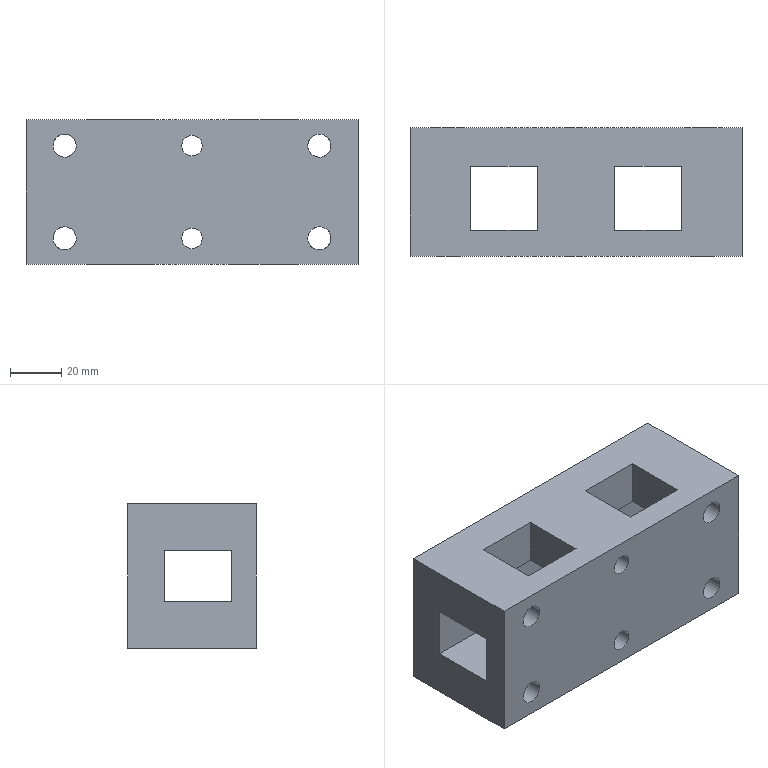Part | STEP file | 车灯-后视镜_id42_x_t | 1 solid | 40 faces | box 129 x 50 x 56 mm | volume 226318 mm3 | plane 30 | cylinder 10 | commonest cylinder face diameters 9 x4 14 x4 8 x2
STEP:
#1=CARTESIAN_POINT('',(65.5,310.,-247.5));
#2=VERTEX_POINT('',#1);
#3=CARTESIAN_POINT('',(65.5,310.,-229.5));
#4=VERTEX_POINT('',#3);
#5=CARTESIAN_POINT('',(65.5,310.,-335.5));
#6=DIRECTION('',(0.,0.,1.));
#7=VECTOR('',#6,1.);
#8=LINE('',#5,#7);
#9=EDGE_CURVE('',#2,#4,#8,.T.);
#10=ORIENTED_EDGE('',*,*,#9,.F.);
#11=CARTESIAN_POINT('',(65.5,285.,-247.5));
#12=VERTEX_POINT('',#11);
#13=CARTESIAN_POINT('',(65.5,292.5,-247.5));
#14=DIRECTION('',(0.,-1.,0.));
#15=VECTOR('',#14,1.);
#16=LINE('',#13,#15);
#17=EDGE_CURVE('',#2,#12,#16,.T.);
#18=ORIENTED_EDGE('',*,*,#17,.T.);
#19=CARTESIAN_POINT('',(65.5,285.,-229.5));
#20=VERTEX_POINT('',#19);
#21=CARTESIAN_POINT('',(65.5,285.,-335.5));
#22=DIRECTION('',(0.,0.,1.));
#23=VECTOR('',#22,1.);
#24=LINE('',#21,#23);
#25=EDGE_CURVE('',#12,#20,#24,.T.);
#26=ORIENTED_EDGE('',*,*,#25,.T.);
#27=CARTESIAN_POINT('',(65.5,292.5,-229.5));
#28=DIRECTION('',(0.,1.,0.));
#29=VECTOR('',#28,1.);
#30=LINE('',#27,#29);
#31=EDGE_CURVE('',#20,#4,#30,.T.);
#32=ORIENTED_EDGE('',*,*,#31,.T.);
#33=EDGE_LOOP('',(#10,#18,#26,#32));
#34=FACE_OUTER_BOUND('',#33,.T.);
#35=CARTESIAN_POINT('',(65.5,292.5,-335.5));
#36=DIRECTION('',(1.,0.,0.));
#37=DIRECTION('',(0.,0.,-1.));
#38=AXIS2_PLACEMENT_3D('',#35,#36,#37);
#39=PLANE('',#38);
#40=ADVANCED_FACE('',(#34),#39,.F.);
#41=ORIENTED_EDGE('',*,*,#25,.F.);
#42=CARTESIAN_POINT('',(39.5,285.,-247.5));
#43=VERTEX_POINT('',#42);
#44=CARTESIAN_POINT('',(52.5,285.,-247.5));
#45=DIRECTION('',(-1.,0.,0.));
#46=VECTOR('',#45,1.);
#47=LINE('',#44,#46);
#48=EDGE_CURVE('',#12,#43,#47,.T.);
#49=ORIENTED_EDGE('',*,*,#48,.T.);
#50=CARTESIAN_POINT('',(39.5,285.,-229.5));
#51=VERTEX_POINT('',#50);
#52=CARTESIAN_POINT('',(39.5,285.,-335.5));
#53=DIRECTION('',(0.,0.,1.));
#54=VECTOR('',#53,1.);
#55=LINE('',#52,#54);
#56=EDGE_CURVE('',#43,#51,#55,.T.);
#57=ORIENTED_EDGE('',*,*,#56,.T.);
#58=CARTESIAN_POINT('',(52.5,285.,-229.5));
#59=DIRECTION('',(1.,0.,0.));
#60=VECTOR('',#59,1.);
#61=LINE('',#58,#60);
#62=EDGE_CURVE('',#51,#20,#61,.T.);
#63=ORIENTED_EDGE('',*,*,#62,.T.);
#64=EDGE_LOOP('',(#41,#49,#57,#63));
#65=FACE_OUTER_BOUND('',#64,.T.);
#66=CARTESIAN_POINT('',(52.5,285.,-335.5));
#67=DIRECTION('',(0.,-1.,0.));
#68=DIRECTION('',(0.,0.,1.));
#69=AXIS2_PLACEMENT_3D('',#66,#67,#68);
#70=PLANE('',#69);
#71=ADVANCED_FACE('',(#65),#70,.F.);
#72=ORIENTED_EDGE('',*,*,#56,.F.);
#73=CARTESIAN_POINT('',(39.5,310.,-247.5));
#74=VERTEX_POINT('',#73);
#75=CARTESIAN_POINT('',(39.5,292.5,-247.5));
#76=DIRECTION('',(0.,1.,0.));
#77=VECTOR('',#76,1.);
#78=LINE('',#75,#77);
#79=EDGE_CURVE('',#43,#74,#78,.T.);
#80=ORIENTED_EDGE('',*,*,#79,.T.);
#81=CARTESIAN_POINT('',(39.5,310.,-229.5));
#82=VERTEX_POINT('',#81);
#83=CARTESIAN_POINT('',(39.5,310.,-335.5));
#84=DIRECTION('',(0.,0.,1.));
#85=VECTOR('',#84,1.);
#86=LINE('',#83,#85);
#87=EDGE_CURVE('',#74,#82,#86,.T.);
#88=ORIENTED_EDGE('',*,*,#87,.T.);
#89=CARTESIAN_POINT('',(39.5,292.5,-229.5));
#90=DIRECTION('',(0.,-1.,0.));
#91=VECTOR('',#90,1.);
#92=LINE('',#89,#91);
#93=EDGE_CURVE('',#82,#51,#92,.T.);
#94=ORIENTED_EDGE('',*,*,#93,.T.);
#95=EDGE_LOOP('',(#72,#80,#88,#94));
#96=FACE_OUTER_BOUND('',#95,.T.);
#97=CARTESIAN_POINT('',(39.5,292.5,-335.5));
#98=DIRECTION('',(-1.,0.,0.));
#99=DIRECTION('',(0.,0.,1.));
#100=AXIS2_PLACEMENT_3D('',#97,#98,#99);
#101=PLANE('',#100);
#102=ADVANCED_FACE('',(#96),#101,.F.);
#103=ORIENTED_EDGE('',*,*,#87,.F.);
#104=CARTESIAN_POINT('',(52.5,310.,-247.5));
#105=DIRECTION('',(1.,0.,0.));
#106=VECTOR('',#105,1.);
#107=LINE('',#104,#106);
#108=EDGE_CURVE('',#74,#2,#107,.T.);
#109=ORIENTED_EDGE('',*,*,#108,.T.);
#110=ORIENTED_EDGE('',*,*,#9,.T.);
#111=CARTESIAN_POINT('',(52.5,310.,-229.5));
#112=DIRECTION('',(-1.,0.,0.));
#113=VECTOR('',#112,1.);
#114=LINE('',#111,#113);
#115=EDGE_CURVE('',#4,#82,#114,.T.);
#116=ORIENTED_EDGE('',*,*,#115,.T.);
#117=EDGE_LOOP('',(#103,#109,#110,#116));
#118=FACE_OUTER_BOUND('',#117,.T.);
#119=CARTESIAN_POINT('',(52.5,310.,-335.5));
#120=DIRECTION('',(0.,1.,0.));
#121=DIRECTION('',(0.,0.,-1.));
#122=AXIS2_PLACEMENT_3D('',#119,#120,#121);
#123=PLANE('',#122);
#124=ADVANCED_FACE('',(#118),#123,.F.);
#125=CARTESIAN_POINT('',(121.5,310.,-247.5));
#126=VERTEX_POINT('',#125);
#127=CARTESIAN_POINT('',(121.5,310.,-229.5));
#128=VERTEX_POINT('',#127);
#129=CARTESIAN_POINT('',(121.5,310.,-335.5));
#130=DIRECTION('',(0.,0.,1.));
#131=VECTOR('',#130,1.);
#132=LINE('',#129,#131);
#133=EDGE_CURVE('',#126,#128,#132,.T.);
#134=ORIENTED_EDGE('',*,*,#133,.F.);
#135=CARTESIAN_POINT('',(121.5,285.,-247.5));
#136=VERTEX_POINT('',#135);
#137=CARTESIAN_POINT('',(121.5,292.5,-247.5));
#138=DIRECTION('',(0.,-1.,0.));
#139=VECTOR('',#138,1.);
#140=LINE('',#137,#139);
#141=EDGE_CURVE('',#126,#136,#140,.T.);
#142=ORIENTED_EDGE('',*,*,#141,.T.);
#143=CARTESIAN_POINT('',(121.5,285.,-229.5));
#144=VERTEX_POINT('',#143);
#145=CARTESIAN_POINT('',(121.5,285.,-335.5));
#146=DIRECTION('',(0.,0.,1.));
#147=VECTOR('',#146,1.);
#148=LINE('',#145,#147);
#149=EDGE_CURVE('',#136,#144,#148,.T.);
#150=ORIENTED_EDGE('',*,*,#149,.T.);
#151=CARTESIAN_POINT('',(121.5,292.5,-229.5));
#152=DIRECTION('',(0.,1.,0.));
#153=VECTOR('',#152,1.);
#154=LINE('',#151,#153);
#155=EDGE_CURVE('',#144,#128,#154,.T.);
#156=ORIENTED_EDGE('',*,*,#155,.T.);
#157=EDGE_LOOP('',(#134,#142,#150,#156));
#158=FACE_OUTER_BOUND('',#157,.T.);
#159=CARTESIAN_POINT('',(121.5,292.5,-335.5));
#160=DIRECTION('',(1.,0.,0.));
#161=DIRECTION('',(0.,0.,-1.));
#162=AXIS2_PLACEMENT_3D('',#159,#160,#161);
#163=PLANE('',#162);
#164=ADVANCED_FACE('',(#158),#163,.F.);
#165=ORIENTED_EDGE('',*,*,#149,.F.);
#166=CARTESIAN_POINT('',(95.5,285.,-247.5));
#167=VERTEX_POINT('',#166);
#168=CARTESIAN_POINT('',(108.5,285.,-247.5));
#169=DIRECTION('',(-1.,0.,0.));
#170=VECTOR('',#169,1.);
#171=LINE('',#168,#170);
#172=EDGE_CURVE('',#136,#167,#171,.T.);
#173=ORIENTED_EDGE('',*,*,#172,.T.);
#174=CARTESIAN_POINT('',(95.5,285.,-229.5));
#175=VERTEX_POINT('',#174);
#176=CARTESIAN_POINT('',(95.5,285.,-335.5));
#177=DIRECTION('',(0.,0.,1.));
#178=VECTOR('',#177,1.);
#179=LINE('',#176,#178);
#180=EDGE_CURVE('',#167,#175,#179,.T.);
#181=ORIENTED_EDGE('',*,*,#180,.T.);
#182=CARTESIAN_POINT('',(108.5,285.,-229.5));
#183=DIRECTION('',(1.,0.,0.));
#184=VECTOR('',#183,1.);
#185=LINE('',#182,#184);
#186=EDGE_CURVE('',#175,#144,#185,.T.);
#187=ORIENTED_EDGE('',*,*,#186,.T.);
#188=EDGE_LOOP('',(#165,#173,#181,#187));
#189=FACE_OUTER_BOUND('',#188,.T.);
#190=CARTESIAN_POINT('',(108.5,285.,-335.5));
#191=DIRECTION('',(0.,-1.,0.));
#192=DIRECTION('',(0.,0.,1.));
#193=AXIS2_PLACEMENT_3D('',#190,#191,#192);
#194=PLANE('',#193);
#195=ADVANCED_FACE('',(#189),#194,.F.);
#196=ORIENTED_EDGE('',*,*,#180,.F.);
#197=CARTESIAN_POINT('',(95.5,310.,-247.5));
#198=VERTEX_POINT('',#197);
#199=CARTESIAN_POINT('',(95.5,292.5,-247.5));
#200=DIRECTION('',(0.,1.,0.));
#201=VECTOR('',#200,1.);
#202=LINE('',#199,#201);
#203=EDGE_CURVE('',#167,#198,#202,.T.);
#204=ORIENTED_EDGE('',*,*,#203,.T.);
#205=CARTESIAN_POINT('',(95.5,310.,-229.5));
#206=VERTEX_POINT('',#205);
#207=CARTESIAN_POINT('',(95.5,310.,-335.5));
#208=DIRECTION('',(0.,0.,1.));
#209=VECTOR('',#208,1.);
#210=LINE('',#207,#209);
#211=EDGE_CURVE('',#198,#206,#210,.T.);
#212=ORIENTED_EDGE('',*,*,#211,.T.);
#213=CARTESIAN_POINT('',(95.5,300.,-229.5));
#214=DIRECTION('',(0.,1.,0.));
#215=VECTOR('',#214,1.);
#216=LINE('',#213,#215);
#217=EDGE_CURVE('',#175,#206,#216,.T.);
#218=ORIENTED_EDGE('',*,*,#217,.F.);
#219=EDGE_LOOP('',(#196,#204,#212,#218));
#220=FACE_OUTER_BOUND('',#219,.T.);
#221=CARTESIAN_POINT('',(95.5,292.5,-335.5));
#222=DIRECTION('',(-1.,0.,0.));
#223=DIRECTION('',(0.,0.,1.));
#224=AXIS2_PLACEMENT_3D('',#221,#222,#223);
#225=PLANE('',#224);
#226=ADVANCED_FACE('',(#220),#225,.F.);
#227=ORIENTED_EDGE('',*,*,#211,.F.);
#228=CARTESIAN_POINT('',(108.5,310.,-247.5));
#229=DIRECTION('',(1.,0.,0.));
#230=VECTOR('',#229,1.);
#231=LINE('',#228,#230);
#232=EDGE_CURVE('',#198,#126,#231,.T.);
#233=ORIENTED_EDGE('',*,*,#232,.T.);
#234=ORIENTED_EDGE('',*,*,#133,.T.);
#235=CARTESIAN_POINT('',(108.5,310.,-229.5));
#236=DIRECTION('',(-1.,0.,0.));
#237=VECTOR('',#236,1.);
#238=LINE('',#235,#237);
#239=EDGE_CURVE('',#128,#206,#238,.T.);
#240=ORIENTED_EDGE('',*,*,#239,.T.);
#241=EDGE_LOOP('',(#227,#233,#234,#240));
#242=FACE_OUTER_BOUND('',#241,.T.);
#243=CARTESIAN_POINT('',(108.5,310.,-335.5));
#244=DIRECTION('',(0.,1.,0.));
#245=DIRECTION('',(0.,0.,-1.));
#246=AXIS2_PLACEMENT_3D('',#243,#244,#245);
#247=PLANE('',#246);
#248=ADVANCED_FACE('',(#242),#247,.F.);
#249=ORIENTED_EDGE('',*,*,#155,.F.);
#250=ORIENTED_EDGE('',*,*,#186,.F.);
#251=ORIENTED_EDGE('',*,*,#217,.T.);
#252=ORIENTED_EDGE('',*,*,#239,.F.);
#253=EDGE_LOOP('',(#249,#250,#251,#252));
#254=FACE_BOUND('',#253,.T.);
#255=ORIENTED_EDGE('',*,*,#31,.F.);
#256=ORIENTED_EDGE('',*,*,#62,.F.);
#257=ORIENTED_EDGE('',*,*,#93,.F.);
#258=ORIENTED_EDGE('',*,*,#115,.F.);
#259=EDGE_LOOP('',(#255,#256,#257,#258));
#260=FACE_BOUND('',#259,.T.);
#261=CARTESIAN_POINT('',(16.,325.,-229.5));
#262=VERTEX_POINT('',#261);
#263=CARTESIAN_POINT('',(145.,325.,-229.5));
#264=VERTEX_POINT('',#263);
#265=CARTESIAN_POINT('',(80.5,325.,-229.5));
#266=DIRECTION('',(1.,0.,0.));
#267=VECTOR('',#266,1.);
#268=LINE('',#265,#267);
#269=EDGE_CURVE('',#262,#264,#268,.T.);
#270=ORIENTED_EDGE('',*,*,#269,.F.);
#271=CARTESIAN_POINT('',(16.,275.,-229.5));
#272=VERTEX_POINT('',#271);
#273=CARTESIAN_POINT('',(16.,300.,-229.5));
#274=DIRECTION('',(0.,1.,0.));
#275=VECTOR('',#274,1.);
#276=LINE('',#273,#275);
#277=EDGE_CURVE('',#272,#262,#276,.T.);
#278=ORIENTED_EDGE('',*,*,#277,.F.);
#279=CARTESIAN_POINT('',(145.,275.,-229.5));
#280=VERTEX_POINT('',#279);
#281=CARTESIAN_POINT('',(80.5,275.,-229.5));
#282=DIRECTION('',(-1.,0.,0.));
#283=VECTOR('',#282,1.);
#284=LINE('',#281,#283);
#285=EDGE_CURVE('',#280,#272,#284,.T.);
#286=ORIENTED_EDGE('',*,*,#285,.F.);
#287=CARTESIAN_POINT('',(145.,300.,-229.5));
#288=DIRECTION('',(0.,-1.,0.));
#289=VECTOR('',#288,1.);
#290=LINE('',#287,#289);
#291=EDGE_CURVE('',#264,#280,#290,.T.);
#292=ORIENTED_EDGE('',*,*,#291,.F.);
#293=EDGE_LOOP('',(#270,#278,#286,#292));
#294=FACE_BOUND('',#293,.T.);
#295=CARTESIAN_POINT('',(80.5,300.,-229.5));
#296=DIRECTION('',(0.,0.,1.));
#297=DIRECTION('',(-1.,0.,0.));
#298=AXIS2_PLACEMENT_3D('',#295,#296,#297);
#299=PLANE('',#298);
#300=ADVANCED_FACE('',(#254,#260,#294),#299,.T.);
#301=CARTESIAN_POINT('',(123.,325.,-239.5));
#302=VERTEX_POINT('',#301);
#303=CARTESIAN_POINT('',(130.,325.,-239.5));
#304=DIRECTION('',(0.,-1.,0.));
#305=DIRECTION('',(-1.,0.,0.));
#306=AXIS2_PLACEMENT_3D('',#303,#304,#305);
#307=CIRCLE('',#306,7.);
#308=EDGE_CURVE('',#302,#302,#307,.T.);
#309=ORIENTED_EDGE('',*,*,#308,.T.);
#310=EDGE_LOOP('',(#309));
#311=FACE_BOUND('',#310,.T.);
#312=CARTESIAN_POINT('',(123.,325.,-275.5));
#313=VERTEX_POINT('',#312);
#314=CARTESIAN_POINT('',(130.,325.,-275.5));
#315=DIRECTION('',(0.,-1.,0.));
#316=DIRECTION('',(-1.,0.,0.));
#317=AXIS2_PLACEMENT_3D('',#314,#315,#316);
#318=CIRCLE('',#317,7.);
#319=EDGE_CURVE('',#313,#313,#318,.T.);
#320=ORIENTED_EDGE('',*,*,#319,.T.);
#321=EDGE_LOOP('',(#320));
#322=FACE_BOUND('',#321,.T.);
#323=CARTESIAN_POINT('',(24.,325.,-275.5));
#324=VERTEX_POINT('',#323);
#325=CARTESIAN_POINT('',(31.,325.,-275.5));
#326=DIRECTION('',(0.,-1.,0.));
#327=DIRECTION('',(-1.,0.,0.));
#328=AXIS2_PLACEMENT_3D('',#325,#326,#327);
#329=CIRCLE('',#328,7.);
#330=EDGE_CURVE('',#324,#324,#329,.T.);
#331=ORIENTED_EDGE('',*,*,#330,.T.);
#332=EDGE_LOOP('',(#331));
#333=FACE_BOUND('',#332,.T.);
#334=CARTESIAN_POINT('',(24.,325.,-239.5));
#335=VERTEX_POINT('',#334);
#336=CARTESIAN_POINT('',(31.,325.,-239.5));
#337=DIRECTION('',(0.,-1.,0.));
#338=DIRECTION('',(-1.,0.,0.));
#339=AXIS2_PLACEMENT_3D('',#336,#337,#338);
#340=CIRCLE('',#339,7.);
#341=EDGE_CURVE('',#335,#335,#340,.T.);
#342=ORIENTED_EDGE('',*,*,#341,.T.);
#343=EDGE_LOOP('',(#342));
#344=FACE_BOUND('',#343,.T.);
#345=CARTESIAN_POINT('',(80.5,325.,-271.5));
#346=VERTEX_POINT('',#345);
#347=CARTESIAN_POINT('',(80.5,325.,-275.5));
#348=DIRECTION('',(0.,-1.,0.));
#349=DIRECTION('',(0.,0.,1.));
#350=AXIS2_PLACEMENT_3D('',#347,#348,#349);
#351=CIRCLE('',#350,4.);
#352=EDGE_CURVE('',#346,#346,#351,.T.);
#353=ORIENTED_EDGE('',*,*,#352,.T.);
#354=EDGE_LOOP('',(#353));
#355=FACE_BOUND('',#354,.T.);
#356=CARTESIAN_POINT('',(80.5,325.,-235.5));
#357=VERTEX_POINT('',#356);
#358=CARTESIAN_POINT('',(80.5,325.,-239.5));
#359=DIRECTION('',(0.,-1.,0.));
#360=DIRECTION('',(0.,0.,1.));
#361=AXIS2_PLACEMENT_3D('',#358,#359,#360);
#362=CIRCLE('',#361,4.);
#363=EDGE_CURVE('',#357,#357,#362,.T.);
#364=ORIENTED_EDGE('',*,*,#363,.T.);
#365=EDGE_LOOP('',(#364));
#366=FACE_BOUND('',#365,.T.);
#367=CARTESIAN_POINT('',(16.,325.,-285.5));
#368=VERTEX_POINT('',#367);
#369=CARTESIAN_POINT('',(16.,325.,-285.5));
#370=DIRECTION('',(0.,0.,1.));
#371=VECTOR('',#370,1.);
#372=LINE('',#369,#371);
#373=EDGE_CURVE('',#368,#262,#372,.T.);
#374=ORIENTED_EDGE('',*,*,#373,.T.);
#375=ORIENTED_EDGE('',*,*,#269,.T.);
#376=CARTESIAN_POINT('',(145.,325.,-285.5));
#377=VERTEX_POINT('',#376);
#378=CARTESIAN_POINT('',(145.,325.,-285.5));
#379=DIRECTION('',(0.,0.,1.));
#380=VECTOR('',#379,1.);
#381=LINE('',#378,#380);
#382=EDGE_CURVE('',#377,#264,#381,.T.);
#383=ORIENTED_EDGE('',*,*,#382,.F.);
#384=CARTESIAN_POINT('',(80.5,325.,-285.5));
#385=DIRECTION('',(-1.,0.,0.));
#386=VECTOR('',#385,1.);
#387=LINE('',#384,#386);
#388=EDGE_CURVE('',#377,#368,#387,.T.);
#389=ORIENTED_EDGE('',*,*,#388,.T.);
#390=EDGE_LOOP('',(#374,#375,#383,#389));
#391=FACE_BOUND('',#390,.T.);
#392=CARTESIAN_POINT('',(80.5,325.,-285.5));
#393=DIRECTION('',(0.,1.,0.));
#394=DIRECTION('',(0.,0.,-1.));
#395=AXIS2_PLACEMENT_3D('',#392,#393,#394);
#396=PLANE('',#395);
#397=ADVANCED_FACE('',(#311,#322,#333,#344,#355,#366,#391),#396,.T.);
#398=CARTESIAN_POINT('',(145.,310.5,-247.5));
#399=VERTEX_POINT('',#398);
#400=CARTESIAN_POINT('',(145.,284.5,-247.5));
#401=VERTEX_POINT('',#400);
#402=CARTESIAN_POINT('',(145.,295.,-247.5));
#403=DIRECTION('',(0.,-1.,0.));
#404=VECTOR('',#403,1.);
#405=LINE('',#402,#404);
#406=EDGE_CURVE('',#399,#401,#405,.T.);
#407=ORIENTED_EDGE('',*,*,#406,.F.);
#408=CARTESIAN_POINT('',(145.,310.5,-267.5));
#409=VERTEX_POINT('',#408);
#410=CARTESIAN_POINT('',(145.,310.5,-268.));
#411=DIRECTION('',(0.,0.,1.));
#412=VECTOR('',#411,1.);
#413=LINE('',#410,#412);
#414=EDGE_CURVE('',#409,#399,#413,.T.);
#415=ORIENTED_EDGE('',*,*,#414,.F.);
#416=CARTESIAN_POINT('',(145.,284.5,-267.5));
#417=VERTEX_POINT('',#416);
#418=CARTESIAN_POINT('',(145.,295.,-267.5));
#419=DIRECTION('',(0.,1.,0.));
#420=VECTOR('',#419,1.);
#421=LINE('',#418,#420);
#422=EDGE_CURVE('',#417,#409,#421,.T.);
#423=ORIENTED_EDGE('',*,*,#422,.F.);
#424=CARTESIAN_POINT('',(145.,284.5,-268.));
#425=DIRECTION('',(0.,0.,1.));
#426=VECTOR('',#425,1.);
#427=LINE('',#424,#426);
#428=EDGE_CURVE('',#417,#401,#427,.T.);
#429=ORIENTED_EDGE('',*,*,#428,.T.);
#430=EDGE_LOOP('',(#407,#415,#423,#429));
#431=FACE_BOUND('',#430,.T.);
#432=ORIENTED_EDGE('',*,*,#382,.T.);
#433=ORIENTED_EDGE('',*,*,#291,.T.);
#434=CARTESIAN_POINT('',(145.,275.,-285.5));
#435=VERTEX_POINT('',#434);
#436=CARTESIAN_POINT('',(145.,275.,-285.5));
#437=DIRECTION('',(0.,0.,1.));
#438=VECTOR('',#437,1.);
#439=LINE('',#436,#438);
#440=EDGE_CURVE('',#435,#280,#439,.T.);
#441=ORIENTED_EDGE('',*,*,#440,.F.);
#442=CARTESIAN_POINT('',(145.,300.,-285.5));
#443=DIRECTION('',(0.,1.,0.));
#444=VECTOR('',#443,1.);
#445=LINE('',#442,#444);
#446=EDGE_CURVE('',#435,#377,#445,.T.);
#447=ORIENTED_EDGE('',*,*,#446,.T.);
#448=EDGE_LOOP('',(#432,#433,#441,#447));
#449=FACE_BOUND('',#448,.T.);
#450=CARTESIAN_POINT('',(145.,300.,-285.5));
#451=DIRECTION('',(1.,0.,0.));
#452=DIRECTION('',(0.,0.,1.));
#453=AXIS2_PLACEMENT_3D('',#450,#451,#452);
#454=PLANE('',#453);
#455=ADVANCED_FACE('',(#431,#449),#454,.T.);
#456=CARTESIAN_POINT('',(125.5,275.,-239.5));
#457=VERTEX_POINT('',#456);
#458=CARTESIAN_POINT('',(130.,275.,-239.5));
#459=DIRECTION('',(0.,1.,0.));
#460=DIRECTION('',(-1.,0.,0.));
#461=AXIS2_PLACEMENT_3D('',#458,#459,#460);
#462=CIRCLE('',#461,4.5);
#463=EDGE_CURVE('',#457,#457,#462,.T.);
#464=ORIENTED_EDGE('',*,*,#463,.T.);
#465=EDGE_LOOP('',(#464));
#466=FACE_BOUND('',#465,.T.);
#467=CARTESIAN_POINT('',(125.5,275.,-275.5));
#468=VERTEX_POINT('',#467);
#469=CARTESIAN_POINT('',(130.,275.,-275.5));
#470=DIRECTION('',(0.,1.,0.));
#471=DIRECTION('',(-1.,0.,0.));
#472=AXIS2_PLACEMENT_3D('',#469,#470,#471);
#473=CIRCLE('',#472,4.5);
#474=EDGE_CURVE('',#468,#468,#473,.T.);
#475=ORIENTED_EDGE('',*,*,#474,.T.);
#476=EDGE_LOOP('',(#475));
#477=FACE_BOUND('',#476,.T.);
#478=CARTESIAN_POINT('',(26.5,275.,-275.5));
#479=VERTEX_POINT('',#478);
#480=CARTESIAN_POINT('',(31.,275.,-275.5));
#481=DIRECTION('',(0.,1.,0.));
#482=DIRECTION('',(-1.,0.,0.));
#483=AXIS2_PLACEMENT_3D('',#480,#481,#482);
#484=CIRCLE('',#483,4.5);
#485=EDGE_CURVE('',#479,#479,#484,.T.);
#486=ORIENTED_EDGE('',*,*,#485,.T.);
#487=EDGE_LOOP('',(#486));
#488=FACE_BOUND('',#487,.T.);
#489=CARTESIAN_POINT('',(26.5,275.,-239.5));
#490=VERTEX_POINT('',#489);
#491=CARTESIAN_POINT('',(31.,275.,-239.5));
#492=DIRECTION('',(0.,1.,0.));
#493=DIRECTION('',(-1.,0.,0.));
#494=AXIS2_PLACEMENT_3D('',#491,#492,#493);
#495=CIRCLE('',#494,4.5);
#496=EDGE_CURVE('',#490,#490,#495,.T.);
#497=ORIENTED_EDGE('',*,*,#496,.T.);
#498=EDGE_LOOP('',(#497));
#499=FACE_BOUND('',#498,.T.);
#500=CARTESIAN_POINT('',(80.5,275.,-271.5));
#501=VERTEX_POINT('',#500);
#502=CARTESIAN_POINT('',(80.5,275.,-275.5));
#503=DIRECTION('',(0.,-1.,0.));
#504=DIRECTION('',(0.,0.,1.));
#505=AXIS2_PLACEMENT_3D('',#502,#503,#504);
#506=CIRCLE('',#505,4.);
#507=EDGE_CURVE('',#501,#501,#506,.T.);
#508=ORIENTED_EDGE('',*,*,#507,.F.);
#509=EDGE_LOOP('',(#508));
#510=FACE_BOUND('',#509,.T.);
#511=CARTESIAN_POINT('',(80.5,275.,-235.5));
#512=VERTEX_POINT('',#511);
#513=CARTESIAN_POINT('',(80.5,275.,-239.5));
#514=DIRECTION('',(0.,-1.,0.));
#515=DIRECTION('',(0.,0.,1.));
#516=AXIS2_PLACEMENT_3D('',#513,#514,#515);
#517=CIRCLE('',#516,4.);
#518=EDGE_CURVE('',#512,#512,#517,.T.);
#519=ORIENTED_EDGE('',*,*,#518,.F.);
#520=EDGE_LOOP('',(#519));
#521=FACE_BOUND('',#520,.T.);
#522=ORIENTED_EDGE('',*,*,#440,.T.);
#523=ORIENTED_EDGE('',*,*,#285,.T.);
#524=CARTESIAN_POINT('',(16.,275.,-285.5));
#525=VERTEX_POINT('',#524);
#526=CARTESIAN_POINT('',(16.,275.,-285.5));
#527=DIRECTION('',(0.,0.,1.));
#528=VECTOR('',#527,1.);
#529=LINE('',#526,#528);
#530=EDGE_CURVE('',#525,#272,#529,.T.);
#531=ORIENTED_EDGE('',*,*,#530,.F.);
#532=CARTESIAN_POINT('',(80.5,275.,-285.5));
#533=DIRECTION('',(1.,0.,0.));
#534=VECTOR('',#533,1.);
#535=LINE('',#532,#534);
#536=EDGE_CURVE('',#525,#435,#535,.T.);
#537=ORIENTED_EDGE('',*,*,#536,.T.);
#538=EDGE_LOOP('',(#522,#523,#531,#537));
#539=FACE_BOUND('',#538,.T.);
#540=CARTESIAN_POINT('',(80.5,275.,-285.5));
#541=DIRECTION('',(0.,-1.,0.));
#542=DIRECTION('',(0.,0.,1.));
#543=AXIS2_PLACEMENT_3D('',#540,#541,#542);
#544=PLANE('',#543);
#545=ADVANCED_FACE('',(#466,#477,#488,#499,#510,#521,#539),#544,.T.);
#546=CARTESIAN_POINT('',(95.5,310.,-285.5));
#547=VERTEX_POINT('',#546);
#548=CARTESIAN_POINT('',(121.5,310.,-285.5));
#549=VERTEX_POINT('',#548);
#550=CARTESIAN_POINT('',(108.5,310.,-285.5));
#551=DIRECTION('',(1.,0.,0.));
#552=VECTOR('',#551,1.);
#553=LINE('',#550,#552);
#554=EDGE_CURVE('',#547,#549,#553,.T.);
#555=ORIENTED_EDGE('',*,*,#554,.F.);
#556=CARTESIAN_POINT('',(95.5,285.,-285.5));
#557=VERTEX_POINT('',#556);
#558=CARTESIAN_POINT('',(95.5,292.5,-285.5));
#559=DIRECTION('',(0.,1.,0.));
#560=VECTOR('',#559,1.);
#561=LINE('',#558,#560);
#562=EDGE_CURVE('',#557,#547,#561,.T.);
#563=ORIENTED_EDGE('',*,*,#562,.F.);
#564=CARTESIAN_POINT('',(121.5,285.,-285.5));
#565=VERTEX_POINT('',#564);
#566=CARTESIAN_POINT('',(108.5,285.,-285.5));
#567=DIRECTION('',(-1.,0.,0.));
#568=VECTOR('',#567,1.);
#569=LINE('',#566,#568);
#570=EDGE_CURVE('',#565,#557,#569,.T.);
#571=ORIENTED_EDGE('',*,*,#570,.F.);
#572=CARTESIAN_POINT('',(121.5,292.5,-285.5));
#573=DIRECTION('',(0.,-1.,0.));
#574=VECTOR('',#573,1.);
#575=LINE('',#572,#574);
#576=EDGE_CURVE('',#549,#565,#575,.T.);
#577=ORIENTED_EDGE('',*,*,#576,.F.);
#578=EDGE_LOOP('',(#555,#563,#571,#577));
#579=FACE_BOUND('',#578,.T.);
#580=ORIENTED_EDGE('',*,*,#446,.F.);
#581=ORIENTED_EDGE('',*,*,#536,.F.);
#582=CARTESIAN_POINT('',(16.,300.,-285.5));
#583=DIRECTION('',(0.,-1.,0.));
#584=VECTOR('',#583,1.);
#585=LINE('',#582,#584);
#586=EDGE_CURVE('',#368,#525,#585,.T.);
#587=ORIENTED_EDGE('',*,*,#586,.F.);
#588=ORIENTED_EDGE('',*,*,#388,.F.);
#589=EDGE_LOOP('',(#580,#581,#587,#588));
#590=FACE_BOUND('',#589,.T.);
#591=CARTESIAN_POINT('',(39.5,310.,-285.5));
#592=VERTEX_POINT('',#591);
#593=CARTESIAN_POINT('',(65.5,310.,-285.5));
#594=VERTEX_POINT('',#593);
#595=CARTESIAN_POINT('',(52.5,310.,-285.5));
#596=DIRECTION('',(1.,0.,0.));
#597=VECTOR('',#596,1.);
#598=LINE('',#595,#597);
#599=EDGE_CURVE('',#592,#594,#598,.T.);
#600=ORIENTED_EDGE('',*,*,#599,.F.);
#601=CARTESIAN_POINT('',(39.5,285.,-285.5));
#602=VERTEX_POINT('',#601);
#603=CARTESIAN_POINT('',(39.5,292.5,-285.5));
#604=DIRECTION('',(0.,1.,0.));
#605=VECTOR('',#604,1.);
#606=LINE('',#603,#605);
#607=EDGE_CURVE('',#602,#592,#606,.T.);
#608=ORIENTED_EDGE('',*,*,#607,.F.);
#609=CARTESIAN_POINT('',(65.5,285.,-285.5));
#610=VERTEX_POINT('',#609);
#611=CARTESIAN_POINT('',(52.5,285.,-285.5));
#612=DIRECTION('',(-1.,0.,0.));
#613=VECTOR('',#612,1.);
#614=LINE('',#611,#613);
#615=EDGE_CURVE('',#610,#602,#614,.T.);
#616=ORIENTED_EDGE('',*,*,#615,.F.);
#617=CARTESIAN_POINT('',(65.5,292.5,-285.5));
#618=DIRECTION('',(0.,-1.,0.));
#619=VECTOR('',#618,1.);
#620=LINE('',#617,#619);
#621=EDGE_CURVE('',#594,#610,#620,.T.);
#622=ORIENTED_EDGE('',*,*,#621,.F.);
#623=EDGE_LOOP('',(#600,#608,#616,#622));
#624=FACE_BOUND('',#623,.T.);
#625=CARTESIAN_POINT('',(80.5,300.,-285.5));
#626=DIRECTION('',(0.,0.,-1.));
#627=DIRECTION('',(1.,0.,0.));
#628=AXIS2_PLACEMENT_3D('',#625,#626,#627);
#629=PLANE('',#628);
#630=ADVANCED_FACE('',(#579,#590,#624),#629,.T.);
#631=CARTESIAN_POINT('',(16.,284.5,-247.5));
#632=VERTEX_POINT('',#631);
#633=CARTESIAN_POINT('',(16.,310.5,-247.5));
#634=VERTEX_POINT('',#633);
#635=CARTESIAN_POINT('',(16.,295.,-247.5));
#636=DIRECTION('',(0.,1.,0.));
#637=VECTOR('',#636,1.);
#638=LINE('',#635,#637);
#639=EDGE_CURVE('',#632,#634,#638,.T.);
#640=ORIENTED_EDGE('',*,*,#639,.F.);
#641=CARTESIAN_POINT('',(16.,284.5,-267.5));
#642=VERTEX_POINT('',#641);
#643=CARTESIAN_POINT('',(16.,284.5,-268.));
#644=DIRECTION('',(0.,0.,1.));
#645=VECTOR('',#644,1.);
#646=LINE('',#643,#645);
#647=EDGE_CURVE('',#642,#632,#646,.T.);
#648=ORIENTED_EDGE('',*,*,#647,.F.);
#649=CARTESIAN_POINT('',(16.,310.5,-267.5));
#650=VERTEX_POINT('',#649);
#651=CARTESIAN_POINT('',(16.,295.,-267.5));
#652=DIRECTION('',(0.,-1.,0.));
#653=VECTOR('',#652,1.);
#654=LINE('',#651,#653);
#655=EDGE_CURVE('',#650,#642,#654,.T.);
#656=ORIENTED_EDGE('',*,*,#655,.F.);
#657=CARTESIAN_POINT('',(16.,310.5,-268.));
#658=DIRECTION('',(0.,0.,1.));
#659=VECTOR('',#658,1.);
#660=LINE('',#657,#659);
#661=EDGE_CURVE('',#650,#634,#660,.T.);
#662=ORIENTED_EDGE('',*,*,#661,.T.);
#663=EDGE_LOOP('',(#640,#648,#656,#662));
#664=FACE_BOUND('',#663,.T.);
#665=ORIENTED_EDGE('',*,*,#586,.T.);
#666=ORIENTED_EDGE('',*,*,#530,.T.);
#667=ORIENTED_EDGE('',*,*,#277,.T.);
#668=ORIENTED_EDGE('',*,*,#373,.F.);
#669=EDGE_LOOP('',(#665,#666,#667,#668));
#670=FACE_BOUND('',#669,.T.);
#671=CARTESIAN_POINT('',(16.,300.,-285.5));
#672=DIRECTION('',(-1.,0.,0.));
#673=DIRECTION('',(0.,0.,-1.));
#674=AXIS2_PLACEMENT_3D('',#671,#672,#673);
#675=PLANE('',#674);
#676=ADVANCED_FACE('',(#664,#670),#675,.T.);
#677=CARTESIAN_POINT('',(65.5,285.,-267.5));
#678=VERTEX_POINT('',#677);
#679=CARTESIAN_POINT('',(65.5,285.,-335.5));
#680=DIRECTION('',(0.,0.,1.));
#681=VECTOR('',#680,1.);
#682=LINE('',#679,#681);
#683=EDGE_CURVE('',#610,#678,#682,.T.);
#684=ORIENTED_EDGE('',*,*,#683,.T.);
#685=CARTESIAN_POINT('',(65.5,310.,-267.5));
#686=VERTEX_POINT('',#685);
#687=CARTESIAN_POINT('',(65.5,292.5,-267.5));
#688=DIRECTION('',(0.,1.,0.));
#689=VECTOR('',#688,1.);
#690=LINE('',#687,#689);
#691=EDGE_CURVE('',#678,#686,#690,.T.);
#692=ORIENTED_EDGE('',*,*,#691,.T.);
#693=CARTESIAN_POINT('',(65.5,310.,-335.5));
#694=DIRECTION('',(0.,0.,1.));
#695=VECTOR('',#694,1.);
#696=LINE('',#693,#695);
#697=EDGE_CURVE('',#594,#686,#696,.T.);
#698=ORIENTED_EDGE('',*,*,#697,.F.);
#699=ORIENTED_EDGE('',*,*,#621,.T.);
#700=EDGE_LOOP('',(#684,#692,#698,#699));
#701=FACE_OUTER_BOUND('',#700,.T.);
#702=CARTESIAN_POINT('',(65.5,292.5,-335.5));
#703=DIRECTION('',(1.,0.,0.));
#704=DIRECTION('',(0.,0.,-1.));
#705=AXIS2_PLACEMENT_3D('',#702,#703,#704);
#706=PLANE('',#705);
#707=ADVANCED_FACE('',(#701),#706,.F.);
#708=CARTESIAN_POINT('',(39.5,285.,-267.5));
#709=VERTEX_POINT('',#708);
#710=CARTESIAN_POINT('',(39.5,285.,-335.5));
#711=DIRECTION('',(0.,0.,1.));
#712=VECTOR('',#711,1.);
#713=LINE('',#710,#712);
#714=EDGE_CURVE('',#602,#709,#713,.T.);
#715=ORIENTED_EDGE('',*,*,#714,.T.);
#716=CARTESIAN_POINT('',(52.5,285.,-267.5));
#717=DIRECTION('',(1.,0.,0.));
#718=VECTOR('',#717,1.);
#719=LINE('',#716,#718);
#720=EDGE_CURVE('',#709,#678,#719,.T.);
#721=ORIENTED_EDGE('',*,*,#720,.T.);
#722=ORIENTED_EDGE('',*,*,#683,.F.);
#723=ORIENTED_EDGE('',*,*,#615,.T.);
#724=EDGE_LOOP('',(#715,#721,#722,#723));
#725=FACE_OUTER_BOUND('',#724,.T.);
#726=CARTESIAN_POINT('',(52.5,285.,-335.5));
#727=DIRECTION('',(0.,-1.,0.));
#728=DIRECTION('',(0.,0.,1.));
#729=AXIS2_PLACEMENT_3D('',#726,#727,#728);
#730=PLANE('',#729);
#731=ADVANCED_FACE('',(#725),#730,.F.);
#732=CARTESIAN_POINT('',(39.5,310.,-267.5));
#733=VERTEX_POINT('',#732);
#734=CARTESIAN_POINT('',(39.5,310.,-335.5));
#735=DIRECTION('',(0.,0.,1.));
#736=VECTOR('',#735,1.);
#737=LINE('',#734,#736);
#738=EDGE_CURVE('',#592,#733,#737,.T.);
#739=ORIENTED_EDGE('',*,*,#738,.T.);
#740=CARTESIAN_POINT('',(39.5,292.5,-267.5));
#741=DIRECTION('',(0.,-1.,0.));
#742=VECTOR('',#741,1.);
#743=LINE('',#740,#742);
#744=EDGE_CURVE('',#733,#709,#743,.T.);
#745=ORIENTED_EDGE('',*,*,#744,.T.);
#746=ORIENTED_EDGE('',*,*,#714,.F.);
#747=ORIENTED_EDGE('',*,*,#607,.T.);
#748=EDGE_LOOP('',(#739,#745,#746,#747));
#749=FACE_OUTER_BOUND('',#748,.T.);
#750=CARTESIAN_POINT('',(39.5,292.5,-335.5));
#751=DIRECTION('',(-1.,0.,0.));
#752=DIRECTION('',(0.,0.,1.));
#753=AXIS2_PLACEMENT_3D('',#750,#751,#752);
#754=PLANE('',#753);
#755=ADVANCED_FACE('',(#749),#754,.F.);
#756=ORIENTED_EDGE('',*,*,#697,.T.);
#757=CARTESIAN_POINT('',(52.5,310.,-267.5));
#758=DIRECTION('',(-1.,0.,0.));
#759=VECTOR('',#758,1.);
#760=LINE('',#757,#759);
#761=EDGE_CURVE('',#686,#733,#760,.T.);
#762=ORIENTED_EDGE('',*,*,#761,.T.);
#763=ORIENTED_EDGE('',*,*,#738,.F.);
#764=ORIENTED_EDGE('',*,*,#599,.T.);
#765=EDGE_LOOP('',(#756,#762,#763,#764));
#766=FACE_OUTER_BOUND('',#765,.T.);
#767=CARTESIAN_POINT('',(52.5,310.,-335.5));
#768=DIRECTION('',(0.,1.,0.));
#769=DIRECTION('',(0.,0.,-1.));
#770=AXIS2_PLACEMENT_3D('',#767,#768,#769);
#771=PLANE('',#770);
#772=ADVANCED_FACE('',(#766),#771,.F.);
#773=CARTESIAN_POINT('',(121.5,285.,-267.5));
#774=VERTEX_POINT('',#773);
#775=CARTESIAN_POINT('',(121.5,285.,-335.5));
#776=DIRECTION('',(0.,0.,1.));
#777=VECTOR('',#776,1.);
#778=LINE('',#775,#777);
#779=EDGE_CURVE('',#565,#774,#778,.T.);
#780=ORIENTED_EDGE('',*,*,#779,.T.);
#781=CARTESIAN_POINT('',(121.5,310.,-267.5));
#782=VERTEX_POINT('',#781);
#783=CARTESIAN_POINT('',(121.5,292.5,-267.5));
#784=DIRECTION('',(0.,1.,0.));
#785=VECTOR('',#784,1.);
#786=LINE('',#783,#785);
#787=EDGE_CURVE('',#774,#782,#786,.T.);
#788=ORIENTED_EDGE('',*,*,#787,.T.);
#789=CARTESIAN_POINT('',(121.5,310.,-335.5));
#790=DIRECTION('',(0.,0.,1.));
#791=VECTOR('',#790,1.);
#792=LINE('',#789,#791);
#793=EDGE_CURVE('',#549,#782,#792,.T.);
#794=ORIENTED_EDGE('',*,*,#793,.F.);
#795=ORIENTED_EDGE('',*,*,#576,.T.);
#796=EDGE_LOOP('',(#780,#788,#794,#795));
#797=FACE_OUTER_BOUND('',#796,.T.);
#798=CARTESIAN_POINT('',(121.5,292.5,-335.5));
#799=DIRECTION('',(1.,0.,0.));
#800=DIRECTION('',(0.,0.,-1.));
#801=AXIS2_PLACEMENT_3D('',#798,#799,#800);
#802=PLANE('',#801);
#803=ADVANCED_FACE('',(#797),#802,.F.);
#804=CARTESIAN_POINT('',(95.5,285.,-267.5));
#805=VERTEX_POINT('',#804);
#806=CARTESIAN_POINT('',(95.5,285.,-335.5));
#807=DIRECTION('',(0.,0.,1.));
#808=VECTOR('',#807,1.);
#809=LINE('',#806,#808);
#810=EDGE_CURVE('',#557,#805,#809,.T.);
#811=ORIENTED_EDGE('',*,*,#810,.T.);
#812=CARTESIAN_POINT('',(108.5,285.,-267.5));
#813=DIRECTION('',(1.,0.,0.));
#814=VECTOR('',#813,1.);
#815=LINE('',#812,#814);
#816=EDGE_CURVE('',#805,#774,#815,.T.);
#817=ORIENTED_EDGE('',*,*,#816,.T.);
#818=ORIENTED_EDGE('',*,*,#779,.F.);
#819=ORIENTED_EDGE('',*,*,#570,.T.);
#820=EDGE_LOOP('',(#811,#817,#818,#819));
#821=FACE_OUTER_BOUND('',#820,.T.);
#822=CARTESIAN_POINT('',(108.5,285.,-335.5));
#823=DIRECTION('',(0.,-1.,0.));
#824=DIRECTION('',(0.,0.,1.));
#825=AXIS2_PLACEMENT_3D('',#822,#823,#824);
#826=PLANE('',#825);
#827=ADVANCED_FACE('',(#821),#826,.F.);
#828=CARTESIAN_POINT('',(95.5,310.,-267.5));
#829=VERTEX_POINT('',#828);
#830=CARTESIAN_POINT('',(95.5,310.,-335.5));
#831=DIRECTION('',(0.,0.,1.));
#832=VECTOR('',#831,1.);
#833=LINE('',#830,#832);
#834=EDGE_CURVE('',#547,#829,#833,.T.);
#835=ORIENTED_EDGE('',*,*,#834,.T.);
#836=CARTESIAN_POINT('',(95.5,292.5,-267.5));
#837=DIRECTION('',(0.,-1.,0.));
#838=VECTOR('',#837,1.);
#839=LINE('',#836,#838);
#840=EDGE_CURVE('',#829,#805,#839,.T.);
#841=ORIENTED_EDGE('',*,*,#840,.T.);
#842=ORIENTED_EDGE('',*,*,#810,.F.);
#843=ORIENTED_EDGE('',*,*,#562,.T.);
#844=EDGE_LOOP('',(#835,#841,#842,#843));
#845=FACE_OUTER_BOUND('',#844,.T.);
#846=CARTESIAN_POINT('',(95.5,292.5,-335.5));
#847=DIRECTION('',(-1.,0.,0.));
#848=DIRECTION('',(0.,0.,1.));
#849=AXIS2_PLACEMENT_3D('',#846,#847,#848);
#850=PLANE('',#849);
#851=ADVANCED_FACE('',(#845),#850,.F.);
#852=ORIENTED_EDGE('',*,*,#793,.T.);
#853=CARTESIAN_POINT('',(108.5,310.,-267.5));
#854=DIRECTION('',(-1.,0.,0.));
#855=VECTOR('',#854,1.);
#856=LINE('',#853,#855);
#857=EDGE_CURVE('',#782,#829,#856,.T.);
#858=ORIENTED_EDGE('',*,*,#857,.T.);
#859=ORIENTED_EDGE('',*,*,#834,.F.);
#860=ORIENTED_EDGE('',*,*,#554,.T.);
#861=EDGE_LOOP('',(#852,#858,#859,#860));
#862=FACE_OUTER_BOUND('',#861,.T.);
#863=CARTESIAN_POINT('',(108.5,310.,-335.5));
#864=DIRECTION('',(0.,1.,0.));
#865=DIRECTION('',(0.,0.,-1.));
#866=AXIS2_PLACEMENT_3D('',#863,#864,#865);
#867=PLANE('',#866);
#868=ADVANCED_FACE('',(#862),#867,.F.);
#869=ORIENTED_EDGE('',*,*,#232,.F.);
#870=ORIENTED_EDGE('',*,*,#203,.F.);
#871=ORIENTED_EDGE('',*,*,#172,.F.);
#872=ORIENTED_EDGE('',*,*,#141,.F.);
#873=EDGE_LOOP('',(#869,#870,#871,#872));
#874=FACE_BOUND('',#873,.T.);
#875=CARTESIAN_POINT('',(80.5,310.5,-247.5));
#876=DIRECTION('',(1.,0.,0.));
#877=VECTOR('',#876,1.);
#878=LINE('',#875,#877);
#879=EDGE_CURVE('',#634,#399,#878,.T.);
#880=ORIENTED_EDGE('',*,*,#879,.T.);
#881=ORIENTED_EDGE('',*,*,#406,.T.);
#882=CARTESIAN_POINT('',(80.5,284.5,-247.5));
#883=DIRECTION('',(-1.,0.,0.));
#884=VECTOR('',#883,1.);
#885=LINE('',#882,#884);
#886=EDGE_CURVE('',#401,#632,#885,.T.);
#887=ORIENTED_EDGE('',*,*,#886,.T.);
#888=ORIENTED_EDGE('',*,*,#639,.T.);
#889=EDGE_LOOP('',(#880,#881,#887,#888));
#890=FACE_BOUND('',#889,.T.);
#891=ORIENTED_EDGE('',*,*,#108,.F.);
#892=ORIENTED_EDGE('',*,*,#79,.F.);
#893=ORIENTED_EDGE('',*,*,#48,.F.);
#894=ORIENTED_EDGE('',*,*,#17,.F.);
#895=EDGE_LOOP('',(#891,#892,#893,#894));
#896=FACE_BOUND('',#895,.T.);
#897=CARTESIAN_POINT('',(80.5,295.,-247.5));
#898=DIRECTION('',(0.,0.,1.));
#899=DIRECTION('',(-1.,0.,0.));
#900=AXIS2_PLACEMENT_3D('',#897,#898,#899);
#901=PLANE('',#900);
#902=ADVANCED_FACE('',(#874,#890,#896),#901,.F.);
#903=ORIENTED_EDGE('',*,*,#816,.F.);
#904=ORIENTED_EDGE('',*,*,#840,.F.);
#905=ORIENTED_EDGE('',*,*,#857,.F.);
#906=ORIENTED_EDGE('',*,*,#787,.F.);
#907=EDGE_LOOP('',(#903,#904,#905,#906));
#908=FACE_BOUND('',#907,.T.);
#909=ORIENTED_EDGE('',*,*,#655,.T.);
#910=CARTESIAN_POINT('',(80.5,284.5,-267.5));
#911=DIRECTION('',(1.,0.,0.));
#912=VECTOR('',#911,1.);
#913=LINE('',#910,#912);
#914=EDGE_CURVE('',#642,#417,#913,.T.);
#915=ORIENTED_EDGE('',*,*,#914,.T.);
#916=ORIENTED_EDGE('',*,*,#422,.T.);
#917=CARTESIAN_POINT('',(80.5,310.5,-267.5));
#918=DIRECTION('',(-1.,0.,0.));
#919=VECTOR('',#918,1.);
#920=LINE('',#917,#919);
#921=EDGE_CURVE('',#409,#650,#920,.T.);
#922=ORIENTED_EDGE('',*,*,#921,.T.);
#923=EDGE_LOOP('',(#909,#915,#916,#922));
#924=FACE_BOUND('',#923,.T.);
#925=ORIENTED_EDGE('',*,*,#720,.F.);
#926=ORIENTED_EDGE('',*,*,#744,.F.);
#927=ORIENTED_EDGE('',*,*,#761,.F.);
#928=ORIENTED_EDGE('',*,*,#691,.F.);
#929=EDGE_LOOP('',(#925,#926,#927,#928));
#930=FACE_BOUND('',#929,.T.);
#931=CARTESIAN_POINT('',(80.5,295.,-267.5));
#932=DIRECTION('',(0.,0.,-1.));
#933=DIRECTION('',(1.,0.,0.));
#934=AXIS2_PLACEMENT_3D('',#931,#932,#933);
#935=PLANE('',#934);
#936=ADVANCED_FACE('',(#908,#924,#930),#935,.F.);
#937=ORIENTED_EDGE('',*,*,#661,.F.);
#938=ORIENTED_EDGE('',*,*,#921,.F.);
#939=ORIENTED_EDGE('',*,*,#414,.T.);
#940=ORIENTED_EDGE('',*,*,#879,.F.);
#941=EDGE_LOOP('',(#937,#938,#939,#940));
#942=FACE_OUTER_BOUND('',#941,.T.);
#943=CARTESIAN_POINT('',(80.5,310.5,-268.));
#944=DIRECTION('',(0.,1.,0.));
#945=DIRECTION('',(0.,0.,-1.));
#946=AXIS2_PLACEMENT_3D('',#943,#944,#945);
#947=PLANE('',#946);
#948=ADVANCED_FACE('',(#942),#947,.F.);
#949=ORIENTED_EDGE('',*,*,#428,.F.);
#950=ORIENTED_EDGE('',*,*,#914,.F.);
#951=ORIENTED_EDGE('',*,*,#647,.T.);
#952=ORIENTED_EDGE('',*,*,#886,.F.);
#953=EDGE_LOOP('',(#949,#950,#951,#952));
#954=FACE_OUTER_BOUND('',#953,.T.);
#955=CARTESIAN_POINT('',(80.5,284.5,-268.));
#956=DIRECTION('',(0.,-1.,0.));
#957=DIRECTION('',(0.,0.,1.));
#958=AXIS2_PLACEMENT_3D('',#955,#956,#957);
#959=PLANE('',#958);
#960=ADVANCED_FACE('',(#954),#959,.F.);
#961=ORIENTED_EDGE('',*,*,#518,.T.);
#962=EDGE_LOOP('',(#961));
#963=FACE_BOUND('',#962,.T.);
#964=ORIENTED_EDGE('',*,*,#363,.F.);
#965=EDGE_LOOP('',(#964));
#966=FACE_BOUND('',#965,.T.);
#967=CARTESIAN_POINT('',(80.5,325.,-239.5));
#968=DIRECTION('',(0.,-1.,0.));
#969=DIRECTION('',(0.,0.,1.));
#970=AXIS2_PLACEMENT_3D('',#967,#968,#969);
#971=CYLINDRICAL_SURFACE('',#970,4.);
#972=ADVANCED_FACE('',(#963,#966),#971,.F.);
#973=ORIENTED_EDGE('',*,*,#507,.T.);
#974=EDGE_LOOP('',(#973));
#975=FACE_BOUND('',#974,.T.);
#976=ORIENTED_EDGE('',*,*,#352,.F.);
#977=EDGE_LOOP('',(#976));
#978=FACE_BOUND('',#977,.T.);
#979=CARTESIAN_POINT('',(80.5,325.,-275.5));
#980=DIRECTION('',(0.,-1.,0.));
#981=DIRECTION('',(0.,0.,1.));
#982=AXIS2_PLACEMENT_3D('',#979,#980,#981);
#983=CYLINDRICAL_SURFACE('',#982,4.);
#984=ADVANCED_FACE('',(#975,#978),#983,.F.);
#985=CARTESIAN_POINT('',(31.,316.,-235.));
#986=VERTEX_POINT('',#985);
#987=CARTESIAN_POINT('',(31.,316.,-239.5));
#988=DIRECTION('',(0.,1.,0.));
#989=DIRECTION('',(0.,0.,1.));
#990=AXIS2_PLACEMENT_3D('',#987,#988,#989);
#991=CIRCLE('',#990,4.5);
#992=EDGE_CURVE('',#986,#986,#991,.T.);
#993=ORIENTED_EDGE('',*,*,#992,.T.);
#994=EDGE_LOOP('',(#993));
#995=FACE_BOUND('',#994,.T.);
#996=ORIENTED_EDGE('',*,*,#496,.F.);
#997=EDGE_LOOP('',(#996));
#998=FACE_BOUND('',#997,.T.);
#999=CARTESIAN_POINT('',(31.,275.5,-239.5));
#1000=DIRECTION('',(0.,1.,0.));
#1001=DIRECTION('',(1.,0.,0.));
#1002=AXIS2_PLACEMENT_3D('',#999,#1000,#1001);
#1003=CYLINDRICAL_SURFACE('',#1002,4.5);
#1004=ADVANCED_FACE('',(#995,#998),#1003,.F.);
#1005=ORIENTED_EDGE('',*,*,#992,.F.);
#1006=EDGE_LOOP('',(#1005));
#1007=FACE_BOUND('',#1006,.T.);
#1008=CARTESIAN_POINT('',(38.,316.,-239.5));
#1009=VERTEX_POINT('',#1008);
#1010=CARTESIAN_POINT('',(31.,316.,-239.5));
#1011=DIRECTION('',(0.,1.,0.));
#1012=DIRECTION('',(1.,0.,0.));
#1013=AXIS2_PLACEMENT_3D('',#1010,#1011,#1012);
#1014=CIRCLE('',#1013,7.);
#1015=EDGE_CURVE('',#1009,#1009,#1014,.T.);
#1016=ORIENTED_EDGE('',*,*,#1015,.T.);
#1017=EDGE_LOOP('',(#1016));
#1018=FACE_BOUND('',#1017,.T.);
#1019=CARTESIAN_POINT('',(31.,316.,-239.5));
#1020=DIRECTION('',(0.,-1.,0.));
#1021=DIRECTION('',(-1.,0.,0.));
#1022=AXIS2_PLACEMENT_3D('',#1019,#1020,#1021);
#1023=PLANE('',#1022);
#1024=ADVANCED_FACE('',(#1007,#1018),#1023,.F.);
#1025=ORIENTED_EDGE('',*,*,#1015,.F.);
#1026=EDGE_LOOP('',(#1025));
#1027=FACE_BOUND('',#1026,.T.);
#1028=ORIENTED_EDGE('',*,*,#341,.F.);
#1029=EDGE_LOOP('',(#1028));
#1030=FACE_BOUND('',#1029,.T.);
#1031=CARTESIAN_POINT('',(31.,325.,-239.5));
#1032=DIRECTION('',(0.,-1.,0.));
#1033=DIRECTION('',(-1.,0.,0.));
#1034=AXIS2_PLACEMENT_3D('',#1031,#1032,#1033);
#1035=CYLINDRICAL_SURFACE('',#1034,7.);
#1036=ADVANCED_FACE('',(#1027,#1030),#1035,.F.);
#1037=CARTESIAN_POINT('',(31.,316.,-271.));
#1038=VERTEX_POINT('',#1037);
#1039=CARTESIAN_POINT('',(31.,316.,-275.5));
#1040=DIRECTION('',(0.,1.,0.));
#1041=DIRECTION('',(0.,0.,1.));
#1042=AXIS2_PLACEMENT_3D('',#1039,#1040,#1041);
#1043=CIRCLE('',#1042,4.5);
#1044=EDGE_CURVE('',#1038,#1038,#1043,.T.);
#1045=ORIENTED_EDGE('',*,*,#1044,.T.);
#1046=EDGE_LOOP('',(#1045));
#1047=FACE_BOUND('',#1046,.T.);
#1048=ORIENTED_EDGE('',*,*,#485,.F.);
#1049=EDGE_LOOP('',(#1048));
#1050=FACE_BOUND('',#1049,.T.);
#1051=CARTESIAN_POINT('',(31.,275.5,-275.5));
#1052=DIRECTION('',(0.,1.,0.));
#1053=DIRECTION('',(1.,0.,0.));
#1054=AXIS2_PLACEMENT_3D('',#1051,#1052,#1053);
#1055=CYLINDRICAL_SURFACE('',#1054,4.5);
#1056=ADVANCED_FACE('',(#1047,#1050),#1055,.F.);
#1057=ORIENTED_EDGE('',*,*,#1044,.F.);
#1058=EDGE_LOOP('',(#1057));
#1059=FACE_BOUND('',#1058,.T.);
#1060=CARTESIAN_POINT('',(38.,316.,-275.5));
#1061=VERTEX_POINT('',#1060);
#1062=CARTESIAN_POINT('',(31.,316.,-275.5));
#1063=DIRECTION('',(0.,1.,0.));
#1064=DIRECTION('',(1.,0.,0.));
#1065=AXIS2_PLACEMENT_3D('',#1062,#1063,#1064);
#1066=CIRCLE('',#1065,7.);
#1067=EDGE_CURVE('',#1061,#1061,#1066,.T.);
#1068=ORIENTED_EDGE('',*,*,#1067,.T.);
#1069=EDGE_LOOP('',(#1068));
#1070=FACE_BOUND('',#1069,.T.);
#1071=CARTESIAN_POINT('',(31.,316.,-275.5));
#1072=DIRECTION('',(0.,-1.,0.));
#1073=DIRECTION('',(-1.,0.,0.));
#1074=AXIS2_PLACEMENT_3D('',#1071,#1072,#1073);
#1075=PLANE('',#1074);
#1076=ADVANCED_FACE('',(#1059,#1070),#1075,.F.);
#1077=ORIENTED_EDGE('',*,*,#1067,.F.);
#1078=EDGE_LOOP('',(#1077));
#1079=FACE_BOUND('',#1078,.T.);
#1080=ORIENTED_EDGE('',*,*,#330,.F.);
#1081=EDGE_LOOP('',(#1080));
#1082=FACE_BOUND('',#1081,.T.);
#1083=CARTESIAN_POINT('',(31.,325.,-275.5));
#1084=DIRECTION('',(0.,-1.,0.));
#1085=DIRECTION('',(-1.,0.,0.));
#1086=AXIS2_PLACEMENT_3D('',#1083,#1084,#1085);
#1087=CYLINDRICAL_SURFACE('',#1086,7.);
#1088=ADVANCED_FACE('',(#1079,#1082),#1087,.F.);
#1089=CARTESIAN_POINT('',(130.,316.,-271.));
#1090=VERTEX_POINT('',#1089);
#1091=CARTESIAN_POINT('',(130.,316.,-275.5));
#1092=DIRECTION('',(0.,1.,0.));
#1093=DIRECTION('',(0.,0.,1.));
#1094=AXIS2_PLACEMENT_3D('',#1091,#1092,#1093);
#1095=CIRCLE('',#1094,4.5);
#1096=EDGE_CURVE('',#1090,#1090,#1095,.T.);
#1097=ORIENTED_EDGE('',*,*,#1096,.T.);
#1098=EDGE_LOOP('',(#1097));
#1099=FACE_BOUND('',#1098,.T.);
#1100=ORIENTED_EDGE('',*,*,#474,.F.);
#1101=EDGE_LOOP('',(#1100));
#1102=FACE_BOUND('',#1101,.T.);
#1103=CARTESIAN_POINT('',(130.,275.5,-275.5));
#1104=DIRECTION('',(0.,1.,0.));
#1105=DIRECTION('',(1.,0.,0.));
#1106=AXIS2_PLACEMENT_3D('',#1103,#1104,#1105);
#1107=CYLINDRICAL_SURFACE('',#1106,4.5);
#1108=ADVANCED_FACE('',(#1099,#1102),#1107,.F.);
#1109=ORIENTED_EDGE('',*,*,#1096,.F.);
#1110=EDGE_LOOP('',(#1109));
#1111=FACE_BOUND('',#1110,.T.);
#1112=CARTESIAN_POINT('',(137.,316.,-275.5));
#1113=VERTEX_POINT('',#1112);
#1114=CARTESIAN_POINT('',(130.,316.,-275.5));
#1115=DIRECTION('',(0.,1.,0.));
#1116=DIRECTION('',(1.,0.,0.));
#1117=AXIS2_PLACEMENT_3D('',#1114,#1115,#1116);
#1118=CIRCLE('',#1117,7.);
#1119=EDGE_CURVE('',#1113,#1113,#1118,.T.);
#1120=ORIENTED_EDGE('',*,*,#1119,.T.);
#1121=EDGE_LOOP('',(#1120));
#1122=FACE_BOUND('',#1121,.T.);
#1123=CARTESIAN_POINT('',(130.,316.,-275.5));
#1124=DIRECTION('',(0.,-1.,0.));
#1125=DIRECTION('',(-1.,0.,0.));
#1126=AXIS2_PLACEMENT_3D('',#1123,#1124,#1125);
#1127=PLANE('',#1126);
#1128=ADVANCED_FACE('',(#1111,#1122),#1127,.F.);
#1129=ORIENTED_EDGE('',*,*,#1119,.F.);
#1130=EDGE_LOOP('',(#1129));
#1131=FACE_BOUND('',#1130,.T.);
#1132=ORIENTED_EDGE('',*,*,#319,.F.);
#1133=EDGE_LOOP('',(#1132));
#1134=FACE_BOUND('',#1133,.T.);
#1135=CARTESIAN_POINT('',(130.,325.,-275.5));
#1136=DIRECTION('',(0.,-1.,0.));
#1137=DIRECTION('',(-1.,0.,0.));
#1138=AXIS2_PLACEMENT_3D('',#1135,#1136,#1137);
#1139=CYLINDRICAL_SURFACE('',#1138,7.);
#1140=ADVANCED_FACE('',(#1131,#1134),#1139,.F.);
#1141=CARTESIAN_POINT('',(130.,316.,-235.));
#1142=VERTEX_POINT('',#1141);
#1143=CARTESIAN_POINT('',(130.,316.,-239.5));
#1144=DIRECTION('',(0.,1.,0.));
#1145=DIRECTION('',(0.,0.,1.));
#1146=AXIS2_PLACEMENT_3D('',#1143,#1144,#1145);
#1147=CIRCLE('',#1146,4.5);
#1148=EDGE_CURVE('',#1142,#1142,#1147,.T.);
#1149=ORIENTED_EDGE('',*,*,#1148,.T.);
#1150=EDGE_LOOP('',(#1149));
#1151=FACE_BOUND('',#1150,.T.);
#1152=ORIENTED_EDGE('',*,*,#463,.F.);
#1153=EDGE_LOOP('',(#1152));
#1154=FACE_BOUND('',#1153,.T.);
#1155=CARTESIAN_POINT('',(130.,275.5,-239.5));
#1156=DIRECTION('',(0.,1.,0.));
#1157=DIRECTION('',(1.,0.,0.));
#1158=AXIS2_PLACEMENT_3D('',#1155,#1156,#1157);
#1159=CYLINDRICAL_SURFACE('',#1158,4.5);
#1160=ADVANCED_FACE('',(#1151,#1154),#1159,.F.);
#1161=ORIENTED_EDGE('',*,*,#1148,.F.);
#1162=EDGE_LOOP('',(#1161));
#1163=FACE_BOUND('',#1162,.T.);
#1164=CARTESIAN_POINT('',(137.,316.,-239.5));
#1165=VERTEX_POINT('',#1164);
#1166=CARTESIAN_POINT('',(130.,316.,-239.5));
#1167=DIRECTION('',(0.,1.,0.));
#1168=DIRECTION('',(1.,0.,0.));
#1169=AXIS2_PLACEMENT_3D('',#1166,#1167,#1168);
#1170=CIRCLE('',#1169,7.);
#1171=EDGE_CURVE('',#1165,#1165,#1170,.T.);
#1172=ORIENTED_EDGE('',*,*,#1171,.T.);
#1173=EDGE_LOOP('',(#1172));
#1174=FACE_BOUND('',#1173,.T.);
#1175=CARTESIAN_POINT('',(130.,316.,-239.5));
#1176=DIRECTION('',(0.,-1.,0.));
#1177=DIRECTION('',(-1.,0.,0.));
#1178=AXIS2_PLACEMENT_3D('',#1175,#1176,#1177);
#1179=PLANE('',#1178);
#1180=ADVANCED_FACE('',(#1163,#1174),#1179,.F.);
#1181=ORIENTED_EDGE('',*,*,#1171,.F.);
#1182=EDGE_LOOP('',(#1181));
#1183=FACE_BOUND('',#1182,.T.);
#1184=ORIENTED_EDGE('',*,*,#308,.F.);
#1185=EDGE_LOOP('',(#1184));
#1186=FACE_BOUND('',#1185,.T.);
#1187=CARTESIAN_POINT('',(130.,325.,-239.5));
#1188=DIRECTION('',(0.,-1.,0.));
#1189=DIRECTION('',(-1.,0.,0.));
#1190=AXIS2_PLACEMENT_3D('',#1187,#1188,#1189);
#1191=CYLINDRICAL_SURFACE('',#1190,7.);
#1192=ADVANCED_FACE('',(#1183,#1186),#1191,.F.);
#1193=CLOSED_SHELL('',(#40,#71,#102,#124,#164,#195,#226,#248,#300,#397,#455,#545,#630,#676,#707,#731,#755,#772,#803,#827,#851,#868,#902,#936,#948,#960,#972,#984,#1004,#1024,#1036,#1056,#1076,#1088,#1108,#1128,#1140,#1160,#1180,#1192));
#1194=MANIFOLD_SOLID_BREP('',#1193);
#1195=(LENGTH_UNIT()NAMED_UNIT(*)SI_UNIT(.MILLI.,.METRE.));
#1196=UNCERTAINTY_MEASURE_WITH_UNIT(LENGTH_MEASURE(0.00002),#1195,'','');
#1197=(NAMED_UNIT(*)PLANE_ANGLE_UNIT()SI_UNIT($,.RADIAN.));
#1198=PLANE_ANGLE_MEASURE_WITH_UNIT(PLANE_ANGLE_MEASURE(0.01745),#1197);
#1199=DIMENSIONAL_EXPONENTS(0.,0.,0.,0.,0.,0.,0.);
#1200=(CONVERSION_BASED_UNIT('DEGREE',#1198)NAMED_UNIT(#1199)PLANE_ANGLE_UNIT());
#1201=(NAMED_UNIT(*)SI_UNIT($,.STERADIAN.)SOLID_ANGLE_UNIT());
#1202=(GEOMETRIC_REPRESENTATION_CONTEXT(3)GLOBAL_UNCERTAINTY_ASSIGNED_CONTEXT((#1196))GLOBAL_UNIT_ASSIGNED_CONTEXT((#1195,#1200,#1201))REPRESENTATION_CONTEXT('',''));
#1203=ADVANCED_BREP_SHAPE_REPRESENTATION('',(#1194),#1202);